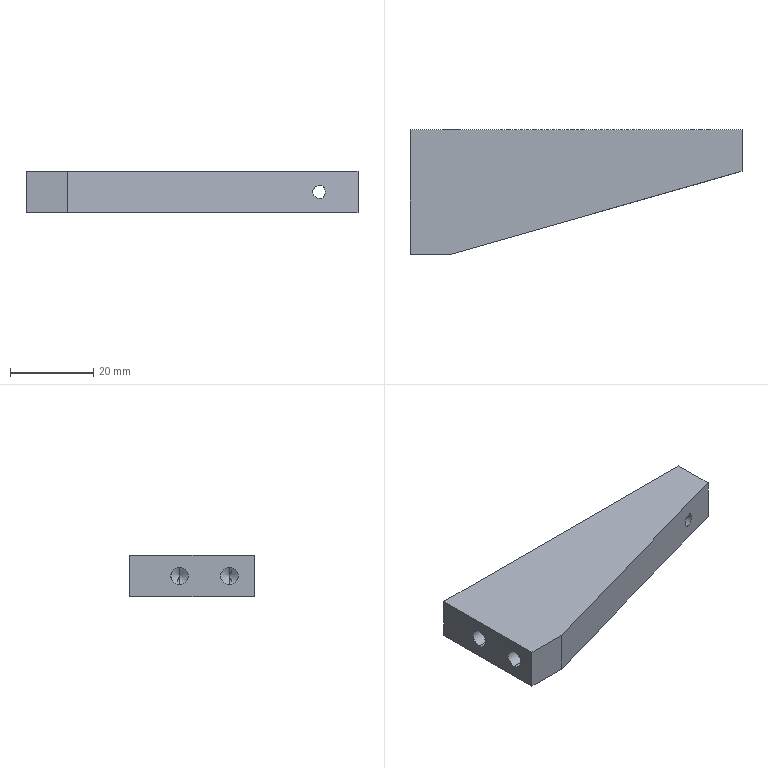Part | NX | features BREP 1 | 1 solid | 33 faces | box 80 x 30 x 10 mm | volume 16150 mm3 | cylinder 14 | cone 12 | plane 7 | commonest cylinder face diameters 4.2 x14
STEP:
#1=CARTESIAN_POINT('',(-30.,2.6,7.1));
#2=VERTEX_POINT('',#1);
#3=CARTESIAN_POINT('',(-29.6,2.6,7.062));
#4=VERTEX_POINT('',#3);
#5=CARTESIAN_POINT('',(-30.,2.6,5.));
#6=DIRECTION('',(0.,1.,0.));
#7=DIRECTION('',(0.,0.,1.));
#8=AXIS2_PLACEMENT_3D('',#5,#6,#7);
#9=CIRCLE('',#8,2.1);
#10=EDGE_CURVE('',#2,#4,#9,.T.);
#11=ORIENTED_EDGE('',*,*,#10,.F.);
#12=CARTESIAN_POINT('',(-30.,3.,7.1));
#13=VERTEX_POINT('',#12);
#14=CARTESIAN_POINT('',(-30.,15.,7.1));
#15=DIRECTION('',(0.,1.,0.));
#16=VECTOR('',#15,1000.);
#17=LINE('',#14,#16);
#18=EDGE_CURVE('',#2,#13,#17,.T.);
#19=ORIENTED_EDGE('',*,*,#18,.T.);
#20=CARTESIAN_POINT('',(-30.,3.,7.1));
#21=CARTESIAN_POINT('',(-29.866,2.866,7.1));
#22=CARTESIAN_POINT('',(-29.732,2.732,7.087));
#23=CARTESIAN_POINT('',(-29.6,2.6,7.062));
#24=(BOUNDED_CURVE()B_SPLINE_CURVE(3,(#20,#21,#22,#23),.UNSPECIFIED.,.F.,.F.)B_SPLINE_CURVE_WITH_KNOTS((4,4),(1.571,1.762),.UNSPECIFIED.)CURVE()GEOMETRIC_REPRESENTATION_ITEM()RATIONAL_B_SPLINE_CURVE((1.,0.9969,0.9969,1.))REPRESENTATION_ITEM(''));
#25=EDGE_CURVE('',#13,#4,#24,.T.);
#26=ORIENTED_EDGE('',*,*,#25,.T.);
#27=EDGE_LOOP('',(#11,#19,#26));
#28=FACE_BOUND('',#27,.T.);
#29=CARTESIAN_POINT('',(-30.,15.,5.));
#30=DIRECTION('',(0.,1.,0.));
#31=DIRECTION('',(0.,0.,1.));
#32=AXIS2_PLACEMENT_3D('',#29,#30,#31);
#33=CYLINDRICAL_SURFACE('',#32,2.1);
#34=ADVANCED_FACE('',(#28),#33,.F.);
#35=CARTESIAN_POINT('',(-30.,2.574,7.056));
#36=VERTEX_POINT('',#35);
#37=CARTESIAN_POINT('',(-30.,2.574,7.056));
#38=CARTESIAN_POINT('',(-29.869,2.574,7.056));
#39=CARTESIAN_POINT('',(-29.735,2.583,7.058));
#40=CARTESIAN_POINT('',(-29.6,2.6,7.062));
#41=B_SPLINE_CURVE_WITH_KNOTS('',3,(#37,#38,#39,#40),.UNSPECIFIED.,.F.,.F.,(4,4),(0.,1.),.UNSPECIFIED.);
#42=EDGE_CURVE('',#4,#36,#41,.F.);
#43=ORIENTED_EDGE('',*,*,#42,.T.);
#44=CARTESIAN_POINT('',(-30.,2.6,7.1));
#45=DIRECTION('',(0.,0.515,0.8572));
#46=VECTOR('',#45,1000.);
#47=LINE('',#44,#46);
#48=EDGE_CURVE('',#36,#2,#47,.T.);
#49=ORIENTED_EDGE('',*,*,#48,.T.);
#50=ORIENTED_EDGE('',*,*,#10,.T.);
#51=EDGE_LOOP('',(#43,#49,#50));
#52=FACE_BOUND('',#51,.T.);
#53=CARTESIAN_POINT('',(-30.,2.6,5.));
#54=DIRECTION('',(0.,1.,0.));
#55=DIRECTION('',(0.,0.,1.));
#56=AXIS2_PLACEMENT_3D('',#53,#54,#55);
#57=CONICAL_SURFACE('',#56,2.1,1.03);
#58=ADVANCED_FACE('',(#52),#57,.F.);
#59=CARTESIAN_POINT('',(-27.6,3.,7.1));
#60=VERTEX_POINT('',#59);
#61=CARTESIAN_POINT('',(-26.338,3.,5.));
#62=VERTEX_POINT('',#61);
#63=CARTESIAN_POINT('',(-27.6,3.,7.1));
#64=DIRECTION('',(-0.515,0.,0.8572));
#65=VECTOR('',#64,1000.);
#66=LINE('',#63,#65);
#67=EDGE_CURVE('',#60,#62,#66,.F.);
#68=ORIENTED_EDGE('',*,*,#67,.T.);
#69=CARTESIAN_POINT('',(-27.6,3.,2.9));
#70=VERTEX_POINT('',#69);
#71=CARTESIAN_POINT('',(-27.6,3.,2.9));
#72=DIRECTION('',(-0.515,0.,-0.8572));
#73=VECTOR('',#72,1000.);
#74=LINE('',#71,#73);
#75=EDGE_CURVE('',#70,#62,#74,.F.);
#76=ORIENTED_EDGE('',*,*,#75,.F.);
#77=CARTESIAN_POINT('',(-27.6,3.,5.));
#78=DIRECTION('',(-1.,0.,0.));
#79=DIRECTION('',(0.,0.,1.));
#80=AXIS2_PLACEMENT_3D('',#77,#78,#79);
#81=CIRCLE('',#80,2.1);
#82=EDGE_CURVE('',#70,#60,#81,.T.);
#83=ORIENTED_EDGE('',*,*,#82,.T.);
#84=EDGE_LOOP('',(#68,#76,#83));
#85=FACE_BOUND('',#84,.T.);
#86=CARTESIAN_POINT('',(-27.6,3.,5.));
#87=DIRECTION('',(-1.,0.,0.));
#88=DIRECTION('',(0.,0.,1.));
#89=AXIS2_PLACEMENT_3D('',#86,#87,#88);
#90=CONICAL_SURFACE('',#89,2.1,1.03);
#91=ADVANCED_FACE('',(#85),#90,.F.);
#92=ORIENTED_EDGE('',*,*,#82,.F.);
#93=CARTESIAN_POINT('',(-30.,3.,2.9));
#94=VERTEX_POINT('',#93);
#95=CARTESIAN_POINT('',(-40.,3.,2.9));
#96=DIRECTION('',(-1.,0.,0.));
#97=VECTOR('',#96,1000.);
#98=LINE('',#95,#97);
#99=EDGE_CURVE('',#94,#70,#98,.F.);
#100=ORIENTED_EDGE('',*,*,#99,.F.);
#101=CARTESIAN_POINT('',(-29.6,2.6,2.938));
#102=VERTEX_POINT('',#101);
#103=CARTESIAN_POINT('',(-29.6,2.6,2.938));
#104=CARTESIAN_POINT('',(-29.732,2.732,2.913));
#105=CARTESIAN_POINT('',(-29.866,2.866,2.9));
#106=CARTESIAN_POINT('',(-30.,3.,2.9));
#107=(BOUNDED_CURVE()B_SPLINE_CURVE(3,(#103,#104,#105,#106),.UNSPECIFIED.,.F.,.F.)B_SPLINE_CURVE_WITH_KNOTS((4,4),(4.521,4.712),.UNSPECIFIED.)CURVE()GEOMETRIC_REPRESENTATION_ITEM()RATIONAL_B_SPLINE_CURVE((1.,0.9969,0.9969,1.))REPRESENTATION_ITEM(''));
#108=EDGE_CURVE('',#102,#94,#107,.T.);
#109=ORIENTED_EDGE('',*,*,#108,.F.);
#110=CARTESIAN_POINT('',(-30.4,2.6,2.938));
#111=VERTEX_POINT('',#110);
#112=CARTESIAN_POINT('',(-29.6,2.6,2.938));
#113=CARTESIAN_POINT('',(-29.872,2.565,2.945));
#114=CARTESIAN_POINT('',(-30.129,2.565,2.945));
#115=CARTESIAN_POINT('',(-30.4,2.6,2.938));
#116=B_SPLINE_CURVE_WITH_KNOTS('',3,(#112,#113,#114,#115),.UNSPECIFIED.,.F.,.F.,(4,4),(0.,1.),.UNSPECIFIED.);
#117=EDGE_CURVE('',#111,#102,#116,.F.);
#118=ORIENTED_EDGE('',*,*,#117,.F.);
#119=CARTESIAN_POINT('',(-30.,3.,2.9));
#120=CARTESIAN_POINT('',(-30.134,2.866,2.9));
#121=CARTESIAN_POINT('',(-30.268,2.732,2.913));
#122=CARTESIAN_POINT('',(-30.4,2.6,2.938));
#123=(BOUNDED_CURVE()B_SPLINE_CURVE(3,(#119,#120,#121,#122),.UNSPECIFIED.,.F.,.F.)B_SPLINE_CURVE_WITH_KNOTS((4,4),(1.571,1.762),.UNSPECIFIED.)CURVE()GEOMETRIC_REPRESENTATION_ITEM()RATIONAL_B_SPLINE_CURVE((1.,0.9969,0.9969,1.))REPRESENTATION_ITEM(''));
#124=EDGE_CURVE('',#94,#111,#123,.T.);
#125=ORIENTED_EDGE('',*,*,#124,.F.);
#126=CARTESIAN_POINT('',(-40.,3.,2.9));
#127=VERTEX_POINT('',#126);
#128=CARTESIAN_POINT('',(-40.,3.,2.9));
#129=DIRECTION('',(-1.,0.,0.));
#130=VECTOR('',#129,1000.);
#131=LINE('',#128,#130);
#132=EDGE_CURVE('',#127,#94,#131,.F.);
#133=ORIENTED_EDGE('',*,*,#132,.F.);
#134=CARTESIAN_POINT('',(-40.,3.,7.1));
#135=VERTEX_POINT('',#134);
#136=CARTESIAN_POINT('',(-40.,3.,5.));
#137=DIRECTION('',(-1.,0.,0.));
#138=DIRECTION('',(0.,0.,1.));
#139=AXIS2_PLACEMENT_3D('',#136,#137,#138);
#140=CIRCLE('',#139,2.1);
#141=EDGE_CURVE('',#127,#135,#140,.T.);
#142=ORIENTED_EDGE('',*,*,#141,.T.);
#143=CARTESIAN_POINT('',(-40.,3.,7.1));
#144=DIRECTION('',(-1.,0.,0.));
#145=VECTOR('',#144,1000.);
#146=LINE('',#143,#145);
#147=EDGE_CURVE('',#135,#13,#146,.F.);
#148=ORIENTED_EDGE('',*,*,#147,.T.);
#149=CARTESIAN_POINT('',(-30.4,2.6,7.062));
#150=VERTEX_POINT('',#149);
#151=CARTESIAN_POINT('',(-30.4,2.6,7.062));
#152=CARTESIAN_POINT('',(-30.268,2.732,7.087));
#153=CARTESIAN_POINT('',(-30.134,2.866,7.1));
#154=CARTESIAN_POINT('',(-30.,3.,7.1));
#155=(BOUNDED_CURVE()B_SPLINE_CURVE(3,(#151,#152,#153,#154),.UNSPECIFIED.,.F.,.F.)B_SPLINE_CURVE_WITH_KNOTS((4,4),(4.521,4.712),.UNSPECIFIED.)CURVE()GEOMETRIC_REPRESENTATION_ITEM()RATIONAL_B_SPLINE_CURVE((1.,0.9969,0.9969,1.))REPRESENTATION_ITEM(''));
#156=EDGE_CURVE('',#150,#13,#155,.T.);
#157=ORIENTED_EDGE('',*,*,#156,.F.);
#158=CARTESIAN_POINT('',(-30.4,2.6,7.062));
#159=CARTESIAN_POINT('',(-30.265,2.583,7.058));
#160=CARTESIAN_POINT('',(-30.131,2.574,7.056));
#161=CARTESIAN_POINT('',(-30.,2.574,7.056));
#162=B_SPLINE_CURVE_WITH_KNOTS('',3,(#158,#159,#160,#161),.UNSPECIFIED.,.F.,.F.,(4,4),(0.,1.),.UNSPECIFIED.);
#163=EDGE_CURVE('',#36,#150,#162,.F.);
#164=ORIENTED_EDGE('',*,*,#163,.F.);
#165=ORIENTED_EDGE('',*,*,#42,.F.);
#166=ORIENTED_EDGE('',*,*,#25,.F.);
#167=CARTESIAN_POINT('',(-40.,3.,7.1));
#168=DIRECTION('',(-1.,0.,0.));
#169=VECTOR('',#168,1000.);
#170=LINE('',#167,#169);
#171=EDGE_CURVE('',#13,#60,#170,.F.);
#172=ORIENTED_EDGE('',*,*,#171,.T.);
#173=EDGE_LOOP('',(#92,#100,#109,#118,#125,#133,#142,#148,#157,#164,#165,#166,#172));
#174=FACE_BOUND('',#173,.T.);
#175=CARTESIAN_POINT('',(-40.,3.,5.));
#176=DIRECTION('',(-1.,0.,0.));
#177=DIRECTION('',(0.,0.,1.));
#178=AXIS2_PLACEMENT_3D('',#175,#176,#177);
#179=CYLINDRICAL_SURFACE('',#178,2.1);
#180=ADVANCED_FACE('',(#174),#179,.F.);
#181=ORIENTED_EDGE('',*,*,#99,.T.);
#182=CARTESIAN_POINT('',(-27.6,3.,5.));
#183=DIRECTION('',(-1.,0.,0.));
#184=DIRECTION('',(0.,0.,1.));
#185=AXIS2_PLACEMENT_3D('',#182,#183,#184);
#186=CIRCLE('',#185,2.1);
#187=EDGE_CURVE('',#60,#70,#186,.T.);
#188=ORIENTED_EDGE('',*,*,#187,.F.);
#189=ORIENTED_EDGE('',*,*,#171,.F.);
#190=CARTESIAN_POINT('',(-30.,3.,2.9));
#191=CARTESIAN_POINT('',(-25.8,7.2,2.9));
#192=CARTESIAN_POINT('',(-25.8,7.2,7.1));
#193=CARTESIAN_POINT('',(-30.,3.,7.1));
#194=(BOUNDED_CURVE()B_SPLINE_CURVE(3,(#190,#191,#192,#193),.UNSPECIFIED.,.F.,.F.)B_SPLINE_CURVE_WITH_KNOTS((4,4),(4.712,7.854),.UNSPECIFIED.)CURVE()GEOMETRIC_REPRESENTATION_ITEM()RATIONAL_B_SPLINE_CURVE((1.,0.3333,0.3333,1.))REPRESENTATION_ITEM(''));
#195=EDGE_CURVE('',#94,#13,#194,.T.);
#196=ORIENTED_EDGE('',*,*,#195,.F.);
#197=EDGE_LOOP('',(#181,#188,#189,#196));
#198=FACE_BOUND('',#197,.T.);
#199=CARTESIAN_POINT('',(-40.,3.,5.));
#200=DIRECTION('',(-1.,0.,0.));
#201=DIRECTION('',(0.,0.,1.));
#202=AXIS2_PLACEMENT_3D('',#199,#200,#201);
#203=CYLINDRICAL_SURFACE('',#202,2.1);
#204=ADVANCED_FACE('',(#198),#203,.F.);
#205=CARTESIAN_POINT('',(-27.6,-9.,2.9));
#206=VERTEX_POINT('',#205);
#207=CARTESIAN_POINT('',(-27.6,-9.,7.1));
#208=VERTEX_POINT('',#207);
#209=CARTESIAN_POINT('',(-27.6,-9.,5.));
#210=DIRECTION('',(-1.,0.,0.));
#211=DIRECTION('',(0.,0.,1.));
#212=AXIS2_PLACEMENT_3D('',#209,#210,#211);
#213=CIRCLE('',#212,2.1);
#214=EDGE_CURVE('',#206,#208,#213,.T.);
#215=ORIENTED_EDGE('',*,*,#214,.F.);
#216=CARTESIAN_POINT('',(-40.,-9.,2.9));
#217=VERTEX_POINT('',#216);
#218=CARTESIAN_POINT('',(-40.,-9.,2.9));
#219=DIRECTION('',(-1.,0.,0.));
#220=VECTOR('',#219,1000.);
#221=LINE('',#218,#220);
#222=EDGE_CURVE('',#217,#206,#221,.F.);
#223=ORIENTED_EDGE('',*,*,#222,.F.);
#224=CARTESIAN_POINT('',(-40.,-9.,7.1));
#225=VERTEX_POINT('',#224);
#226=CARTESIAN_POINT('',(-40.,-9.,5.));
#227=DIRECTION('',(-1.,0.,0.));
#228=DIRECTION('',(0.,0.,1.));
#229=AXIS2_PLACEMENT_3D('',#226,#227,#228);
#230=CIRCLE('',#229,2.1);
#231=EDGE_CURVE('',#217,#225,#230,.T.);
#232=ORIENTED_EDGE('',*,*,#231,.T.);
#233=CARTESIAN_POINT('',(-40.,-9.,7.1));
#234=DIRECTION('',(-1.,0.,0.));
#235=VECTOR('',#234,1000.);
#236=LINE('',#233,#235);
#237=EDGE_CURVE('',#225,#208,#236,.F.);
#238=ORIENTED_EDGE('',*,*,#237,.T.);
#239=EDGE_LOOP('',(#215,#223,#232,#238));
#240=FACE_BOUND('',#239,.T.);
#241=CARTESIAN_POINT('',(-40.,-9.,5.));
#242=DIRECTION('',(-1.,0.,0.));
#243=DIRECTION('',(0.,0.,1.));
#244=AXIS2_PLACEMENT_3D('',#241,#242,#243);
#245=CYLINDRICAL_SURFACE('',#244,2.1);
#246=ADVANCED_FACE('',(#240),#245,.F.);
#247=CARTESIAN_POINT('',(-26.338,-9.,5.));
#248=VERTEX_POINT('',#247);
#249=CARTESIAN_POINT('',(-27.6,-9.,7.1));
#250=DIRECTION('',(-0.515,0.,0.8572));
#251=VECTOR('',#250,1000.);
#252=LINE('',#249,#251);
#253=EDGE_CURVE('',#208,#248,#252,.F.);
#254=ORIENTED_EDGE('',*,*,#253,.T.);
#255=CARTESIAN_POINT('',(-27.6,-9.,2.9));
#256=DIRECTION('',(-0.515,0.,-0.8572));
#257=VECTOR('',#256,1000.);
#258=LINE('',#255,#257);
#259=EDGE_CURVE('',#206,#248,#258,.F.);
#260=ORIENTED_EDGE('',*,*,#259,.F.);
#261=ORIENTED_EDGE('',*,*,#214,.T.);
#262=EDGE_LOOP('',(#254,#260,#261));
#263=FACE_BOUND('',#262,.T.);
#264=CARTESIAN_POINT('',(-27.6,-9.,5.));
#265=DIRECTION('',(-1.,0.,0.));
#266=DIRECTION('',(0.,0.,1.));
#267=AXIS2_PLACEMENT_3D('',#264,#265,#266);
#268=CONICAL_SURFACE('',#267,2.1,1.03);
#269=ADVANCED_FACE('',(#263),#268,.F.);
#270=CARTESIAN_POINT('',(0.,2.6,2.9));
#271=VERTEX_POINT('',#270);
#272=CARTESIAN_POINT('',(0.,2.6,7.1));
#273=VERTEX_POINT('',#272);
#274=CARTESIAN_POINT('',(0.,2.6,5.));
#275=DIRECTION('',(0.,1.,0.));
#276=DIRECTION('',(0.,0.,1.));
#277=AXIS2_PLACEMENT_3D('',#274,#275,#276);
#278=CIRCLE('',#277,2.1);
#279=EDGE_CURVE('',#271,#273,#278,.T.);
#280=ORIENTED_EDGE('',*,*,#279,.F.);
#281=CARTESIAN_POINT('',(0.,15.,2.9));
#282=VERTEX_POINT('',#281);
#283=CARTESIAN_POINT('',(0.,15.,2.9));
#284=DIRECTION('',(0.,1.,0.));
#285=VECTOR('',#284,1000.);
#286=LINE('',#283,#285);
#287=EDGE_CURVE('',#282,#271,#286,.F.);
#288=ORIENTED_EDGE('',*,*,#287,.F.);
#289=CARTESIAN_POINT('',(0.,15.,7.1));
#290=VERTEX_POINT('',#289);
#291=CARTESIAN_POINT('',(0.,15.,5.));
#292=DIRECTION('',(0.,1.,0.));
#293=DIRECTION('',(0.,0.,1.));
#294=AXIS2_PLACEMENT_3D('',#291,#292,#293);
#295=CIRCLE('',#294,2.1);
#296=EDGE_CURVE('',#282,#290,#295,.T.);
#297=ORIENTED_EDGE('',*,*,#296,.T.);
#298=CARTESIAN_POINT('',(0.,15.,7.1));
#299=DIRECTION('',(0.,1.,0.));
#300=VECTOR('',#299,1000.);
#301=LINE('',#298,#300);
#302=EDGE_CURVE('',#290,#273,#301,.F.);
#303=ORIENTED_EDGE('',*,*,#302,.T.);
#304=EDGE_LOOP('',(#280,#288,#297,#303));
#305=FACE_BOUND('',#304,.T.);
#306=CARTESIAN_POINT('',(0.,15.,5.));
#307=DIRECTION('',(0.,1.,0.));
#308=DIRECTION('',(0.,0.,1.));
#309=AXIS2_PLACEMENT_3D('',#306,#307,#308);
#310=CYLINDRICAL_SURFACE('',#309,2.1);
#311=ADVANCED_FACE('',(#305),#310,.F.);
#312=CARTESIAN_POINT('',(0.,1.338,5.));
#313=VERTEX_POINT('',#312);
#314=CARTESIAN_POINT('',(0.,2.6,7.1));
#315=DIRECTION('',(0.,0.515,0.8572));
#316=VECTOR('',#315,1000.);
#317=LINE('',#314,#316);
#318=EDGE_CURVE('',#273,#313,#317,.F.);
#319=ORIENTED_EDGE('',*,*,#318,.T.);
#320=CARTESIAN_POINT('',(0.,2.6,2.9));
#321=DIRECTION('',(0.,0.515,-0.8572));
#322=VECTOR('',#321,1000.);
#323=LINE('',#320,#322);
#324=EDGE_CURVE('',#271,#313,#323,.F.);
#325=ORIENTED_EDGE('',*,*,#324,.F.);
#326=ORIENTED_EDGE('',*,*,#279,.T.);
#327=EDGE_LOOP('',(#319,#325,#326));
#328=FACE_BOUND('',#327,.T.);
#329=CARTESIAN_POINT('',(0.,2.6,5.));
#330=DIRECTION('',(0.,1.,0.));
#331=DIRECTION('',(0.,0.,1.));
#332=AXIS2_PLACEMENT_3D('',#329,#330,#331);
#333=CONICAL_SURFACE('',#332,2.1,1.03);
#334=ADVANCED_FACE('',(#328),#333,.F.);
#335=CARTESIAN_POINT('',(30.,2.6,2.9));
#336=VERTEX_POINT('',#335);
#337=CARTESIAN_POINT('',(30.,2.6,7.1));
#338=VERTEX_POINT('',#337);
#339=CARTESIAN_POINT('',(30.,2.6,5.));
#340=DIRECTION('',(0.,1.,0.));
#341=DIRECTION('',(0.,0.,1.));
#342=AXIS2_PLACEMENT_3D('',#339,#340,#341);
#343=CIRCLE('',#342,2.1);
#344=EDGE_CURVE('',#336,#338,#343,.T.);
#345=ORIENTED_EDGE('',*,*,#344,.F.);
#346=CARTESIAN_POINT('',(30.,15.,2.9));
#347=VERTEX_POINT('',#346);
#348=CARTESIAN_POINT('',(30.,15.,2.9));
#349=DIRECTION('',(0.,1.,0.));
#350=VECTOR('',#349,1000.);
#351=LINE('',#348,#350);
#352=EDGE_CURVE('',#347,#336,#351,.F.);
#353=ORIENTED_EDGE('',*,*,#352,.F.);
#354=CARTESIAN_POINT('',(30.,15.,7.1));
#355=VERTEX_POINT('',#354);
#356=CARTESIAN_POINT('',(30.,15.,5.));
#357=DIRECTION('',(0.,1.,0.));
#358=DIRECTION('',(0.,0.,1.));
#359=AXIS2_PLACEMENT_3D('',#356,#357,#358);
#360=CIRCLE('',#359,2.1);
#361=EDGE_CURVE('',#347,#355,#360,.T.);
#362=ORIENTED_EDGE('',*,*,#361,.T.);
#363=CARTESIAN_POINT('',(30.,15.,7.1));
#364=DIRECTION('',(0.,1.,0.));
#365=VECTOR('',#364,1000.);
#366=LINE('',#363,#365);
#367=EDGE_CURVE('',#355,#338,#366,.F.);
#368=ORIENTED_EDGE('',*,*,#367,.T.);
#369=EDGE_LOOP('',(#345,#353,#362,#368));
#370=FACE_BOUND('',#369,.T.);
#371=CARTESIAN_POINT('',(30.,15.,5.));
#372=DIRECTION('',(0.,1.,0.));
#373=DIRECTION('',(0.,0.,1.));
#374=AXIS2_PLACEMENT_3D('',#371,#372,#373);
#375=CYLINDRICAL_SURFACE('',#374,2.1);
#376=ADVANCED_FACE('',(#370),#375,.F.);
#377=CARTESIAN_POINT('',(30.,2.143,3.661));
#378=VERTEX_POINT('',#377);
#379=CARTESIAN_POINT('',(30.,2.143,6.339));
#380=VERTEX_POINT('',#379);
#381=CARTESIAN_POINT('',(30.,2.143,3.661));
#382=CARTESIAN_POINT('',(28.627,1.751,4.314));
#383=CARTESIAN_POINT('',(28.627,1.751,5.686));
#384=CARTESIAN_POINT('',(30.,2.143,6.339));
#385=(BOUNDED_CURVE()B_SPLINE_CURVE(3,(#381,#382,#383,#384),.UNSPECIFIED.,.F.,.F.)B_SPLINE_CURVE_WITH_KNOTS((4,4),(2.066,4.217),.UNSPECIFIED.)CURVE()GEOMETRIC_REPRESENTATION_ITEM()RATIONAL_B_SPLINE_CURVE((1.,0.6503,0.6503,1.))REPRESENTATION_ITEM(''));
#386=EDGE_CURVE('',#378,#380,#385,.T.);
#387=ORIENTED_EDGE('',*,*,#386,.F.);
#388=CARTESIAN_POINT('',(30.,2.6,2.9));
#389=DIRECTION('',(0.,0.515,-0.8572));
#390=VECTOR('',#389,1000.);
#391=LINE('',#388,#390);
#392=EDGE_CURVE('',#378,#336,#391,.T.);
#393=ORIENTED_EDGE('',*,*,#392,.T.);
#394=ORIENTED_EDGE('',*,*,#344,.T.);
#395=CARTESIAN_POINT('',(30.,2.6,7.1));
#396=DIRECTION('',(0.,0.515,0.8572));
#397=VECTOR('',#396,1000.);
#398=LINE('',#395,#397);
#399=EDGE_CURVE('',#380,#338,#398,.T.);
#400=ORIENTED_EDGE('',*,*,#399,.F.);
#401=EDGE_LOOP('',(#387,#393,#394,#400));
#402=FACE_BOUND('',#401,.T.);
#403=CARTESIAN_POINT('',(30.,2.6,5.));
#404=DIRECTION('',(0.,1.,0.));
#405=DIRECTION('',(0.,0.,1.));
#406=AXIS2_PLACEMENT_3D('',#403,#404,#405);
#407=CONICAL_SURFACE('',#406,2.1,1.03);
#408=ADVANCED_FACE('',(#402),#407,.F.);
#409=CARTESIAN_POINT('',(31.6,2.6,6.36));
#410=VERTEX_POINT('',#409);
#411=CARTESIAN_POINT('',(30.,2.143,6.339));
#412=CARTESIAN_POINT('',(30.508,2.288,6.581));
#413=CARTESIAN_POINT('',(31.084,2.453,6.588));
#414=CARTESIAN_POINT('',(31.6,2.6,6.36));
#415=(BOUNDED_CURVE()B_SPLINE_CURVE(3,(#411,#412,#413,#414),.UNSPECIFIED.,.F.,.F.)B_SPLINE_CURVE_WITH_KNOTS((4,4),(4.217,5.178),.UNSPECIFIED.)CURVE()GEOMETRIC_REPRESENTATION_ITEM()RATIONAL_B_SPLINE_CURVE((1.,0.9245,0.9245,1.))REPRESENTATION_ITEM(''));
#416=EDGE_CURVE('',#380,#410,#415,.T.);
#417=ORIENTED_EDGE('',*,*,#416,.F.);
#418=ORIENTED_EDGE('',*,*,#399,.T.);
#419=CARTESIAN_POINT('',(30.,2.6,5.));
#420=DIRECTION('',(0.,1.,0.));
#421=DIRECTION('',(0.,0.,1.));
#422=AXIS2_PLACEMENT_3D('',#419,#420,#421);
#423=CIRCLE('',#422,2.1);
#424=EDGE_CURVE('',#338,#410,#423,.T.);
#425=ORIENTED_EDGE('',*,*,#424,.T.);
#426=EDGE_LOOP('',(#417,#418,#425));
#427=FACE_BOUND('',#426,.T.);
#428=CARTESIAN_POINT('',(30.,2.6,5.));
#429=DIRECTION('',(0.,1.,0.));
#430=DIRECTION('',(0.,0.,1.));
#431=AXIS2_PLACEMENT_3D('',#428,#429,#430);
#432=CONICAL_SURFACE('',#431,2.1,1.03);
#433=ADVANCED_FACE('',(#427),#432,.F.);
#434=CARTESIAN_POINT('',(-30.,3.,7.1));
#435=CARTESIAN_POINT('',(-34.2,7.2,7.1));
#436=CARTESIAN_POINT('',(-34.2,7.2,2.9));
#437=CARTESIAN_POINT('',(-30.,3.,2.9));
#438=(BOUNDED_CURVE()B_SPLINE_CURVE(3,(#434,#435,#436,#437),.UNSPECIFIED.,.F.,.F.)B_SPLINE_CURVE_WITH_KNOTS((4,4),(4.712,7.854),.UNSPECIFIED.)CURVE()GEOMETRIC_REPRESENTATION_ITEM()RATIONAL_B_SPLINE_CURVE((1.,0.3333,0.3333,1.))REPRESENTATION_ITEM(''));
#439=EDGE_CURVE('',#13,#94,#438,.T.);
#440=ORIENTED_EDGE('',*,*,#439,.T.);
#441=CARTESIAN_POINT('',(-30.,15.,2.9));
#442=VERTEX_POINT('',#441);
#443=CARTESIAN_POINT('',(-30.,15.,2.9));
#444=DIRECTION('',(0.,1.,0.));
#445=VECTOR('',#444,1000.);
#446=LINE('',#443,#445);
#447=EDGE_CURVE('',#442,#94,#446,.F.);
#448=ORIENTED_EDGE('',*,*,#447,.F.);
#449=CARTESIAN_POINT('',(-30.,15.,7.1));
#450=VERTEX_POINT('',#449);
#451=CARTESIAN_POINT('',(-30.,15.,5.));
#452=DIRECTION('',(0.,1.,0.));
#453=DIRECTION('',(0.,0.,1.));
#454=AXIS2_PLACEMENT_3D('',#451,#452,#453);
#455=CIRCLE('',#454,2.1);
#456=EDGE_CURVE('',#442,#450,#455,.T.);
#457=ORIENTED_EDGE('',*,*,#456,.T.);
#458=CARTESIAN_POINT('',(-30.,15.,7.1));
#459=DIRECTION('',(0.,1.,0.));
#460=VECTOR('',#459,1000.);
#461=LINE('',#458,#460);
#462=EDGE_CURVE('',#450,#13,#461,.F.);
#463=ORIENTED_EDGE('',*,*,#462,.T.);
#464=EDGE_LOOP('',(#440,#448,#457,#463));
#465=FACE_BOUND('',#464,.T.);
#466=CARTESIAN_POINT('',(-30.,15.,5.));
#467=DIRECTION('',(0.,1.,0.));
#468=DIRECTION('',(0.,0.,1.));
#469=AXIS2_PLACEMENT_3D('',#466,#467,#468);
#470=CYLINDRICAL_SURFACE('',#469,2.1);
#471=ADVANCED_FACE('',(#465),#470,.F.);
#472=ORIENTED_EDGE('',*,*,#447,.T.);
#473=ORIENTED_EDGE('',*,*,#195,.T.);
#474=ORIENTED_EDGE('',*,*,#462,.F.);
#475=CARTESIAN_POINT('',(-30.,15.,5.));
#476=DIRECTION('',(0.,1.,0.));
#477=DIRECTION('',(0.,0.,1.));
#478=AXIS2_PLACEMENT_3D('',#475,#476,#477);
#479=CIRCLE('',#478,2.1);
#480=EDGE_CURVE('',#450,#442,#479,.T.);
#481=ORIENTED_EDGE('',*,*,#480,.T.);
#482=EDGE_LOOP('',(#472,#473,#474,#481));
#483=FACE_BOUND('',#482,.T.);
#484=CARTESIAN_POINT('',(-30.,15.,5.));
#485=DIRECTION('',(0.,1.,0.));
#486=DIRECTION('',(0.,0.,1.));
#487=AXIS2_PLACEMENT_3D('',#484,#485,#486);
#488=CYLINDRICAL_SURFACE('',#487,2.1);
#489=ADVANCED_FACE('',(#483),#488,.F.);
#490=CARTESIAN_POINT('',(-40.,15.,0.));
#491=VERTEX_POINT('',#490);
#492=CARTESIAN_POINT('',(-40.,-15.,0.));
#493=VERTEX_POINT('',#492);
#494=CARTESIAN_POINT('',(-40.,-15.,0.));
#495=DIRECTION('',(0.,-1.,0.));
#496=VECTOR('',#495,1000.);
#497=LINE('',#494,#496);
#498=EDGE_CURVE('',#491,#493,#497,.T.);
#499=ORIENTED_EDGE('',*,*,#498,.T.);
#500=CARTESIAN_POINT('',(-40.,-15.,10.));
#501=VERTEX_POINT('',#500);
#502=CARTESIAN_POINT('',(-40.,-15.,10.));
#503=DIRECTION('',(0.,0.,-1.));
#504=VECTOR('',#503,1000.);
#505=LINE('',#502,#504);
#506=EDGE_CURVE('',#501,#493,#505,.T.);
#507=ORIENTED_EDGE('',*,*,#506,.F.);
#508=CARTESIAN_POINT('',(-40.,15.,10.));
#509=VERTEX_POINT('',#508);
#510=CARTESIAN_POINT('',(-40.,-15.,10.));
#511=DIRECTION('',(0.,-1.,0.));
#512=VECTOR('',#511,1000.);
#513=LINE('',#510,#512);
#514=EDGE_CURVE('',#509,#501,#513,.T.);
#515=ORIENTED_EDGE('',*,*,#514,.F.);
#516=CARTESIAN_POINT('',(-40.,15.,10.));
#517=DIRECTION('',(0.,0.,-1.));
#518=VECTOR('',#517,1000.);
#519=LINE('',#516,#518);
#520=EDGE_CURVE('',#509,#491,#519,.T.);
#521=ORIENTED_EDGE('',*,*,#520,.T.);
#522=EDGE_LOOP('',(#499,#507,#515,#521));
#523=FACE_BOUND('',#522,.T.);
#524=CARTESIAN_POINT('',(-40.,3.,5.));
#525=DIRECTION('',(-1.,0.,0.));
#526=DIRECTION('',(0.,0.,1.));
#527=AXIS2_PLACEMENT_3D('',#524,#525,#526);
#528=CIRCLE('',#527,2.1);
#529=EDGE_CURVE('',#135,#127,#528,.T.);
#530=ORIENTED_EDGE('',*,*,#529,.F.);
#531=ORIENTED_EDGE('',*,*,#141,.F.);
#532=EDGE_LOOP('',(#530,#531));
#533=FACE_BOUND('',#532,.T.);
#534=CARTESIAN_POINT('',(-40.,-9.,5.));
#535=DIRECTION('',(-1.,0.,0.));
#536=DIRECTION('',(0.,0.,1.));
#537=AXIS2_PLACEMENT_3D('',#534,#535,#536);
#538=CIRCLE('',#537,2.1);
#539=EDGE_CURVE('',#225,#217,#538,.T.);
#540=ORIENTED_EDGE('',*,*,#539,.F.);
#541=ORIENTED_EDGE('',*,*,#231,.F.);
#542=EDGE_LOOP('',(#540,#541));
#543=FACE_BOUND('',#542,.T.);
#544=CARTESIAN_POINT('',(-40.,-15.,10.));
#545=DIRECTION('',(1.,0.,0.));
#546=DIRECTION('',(0.,1.,0.));
#547=AXIS2_PLACEMENT_3D('',#544,#545,#546);
#548=PLANE('',#547);
#549=ADVANCED_FACE('',(#523,#533,#543),#548,.F.);
#550=CARTESIAN_POINT('',(-30.,-15.,0.));
#551=VERTEX_POINT('',#550);
#552=CARTESIAN_POINT('',(-40.,-15.,0.));
#553=DIRECTION('',(1.,0.,0.));
#554=VECTOR('',#553,1000.);
#555=LINE('',#552,#554);
#556=EDGE_CURVE('',#493,#551,#555,.T.);
#557=ORIENTED_EDGE('',*,*,#556,.T.);
#558=CARTESIAN_POINT('',(-30.,-15.,10.));
#559=VERTEX_POINT('',#558);
#560=CARTESIAN_POINT('',(-30.,-15.,10.));
#561=DIRECTION('',(0.,0.,-1.));
#562=VECTOR('',#561,1000.);
#563=LINE('',#560,#562);
#564=EDGE_CURVE('',#559,#551,#563,.T.);
#565=ORIENTED_EDGE('',*,*,#564,.F.);
#566=CARTESIAN_POINT('',(-40.,-15.,10.));
#567=DIRECTION('',(1.,0.,0.));
#568=VECTOR('',#567,1000.);
#569=LINE('',#566,#568);
#570=EDGE_CURVE('',#501,#559,#569,.T.);
#571=ORIENTED_EDGE('',*,*,#570,.F.);
#572=ORIENTED_EDGE('',*,*,#506,.T.);
#573=EDGE_LOOP('',(#557,#565,#571,#572));
#574=FACE_BOUND('',#573,.T.);
#575=CARTESIAN_POINT('',(-40.,-15.,10.));
#576=DIRECTION('',(0.,1.,0.));
#577=DIRECTION('',(1.,0.,0.));
#578=AXIS2_PLACEMENT_3D('',#575,#576,#577);
#579=PLANE('',#578);
#580=ADVANCED_FACE('',(#574),#579,.F.);
#581=CARTESIAN_POINT('',(40.,5.,0.));
#582=VERTEX_POINT('',#581);
#583=CARTESIAN_POINT('',(-30.,-15.,0.));
#584=DIRECTION('',(0.9615,0.2747,0.));
#585=VECTOR('',#584,1000.);
#586=LINE('',#583,#585);
#587=EDGE_CURVE('',#551,#582,#586,.T.);
#588=ORIENTED_EDGE('',*,*,#587,.T.);
#589=CARTESIAN_POINT('',(40.,5.,10.));
#590=VERTEX_POINT('',#589);
#591=CARTESIAN_POINT('',(40.,5.,10.));
#592=DIRECTION('',(0.,0.,-1.));
#593=VECTOR('',#592,1000.);
#594=LINE('',#591,#593);
#595=EDGE_CURVE('',#590,#582,#594,.T.);
#596=ORIENTED_EDGE('',*,*,#595,.F.);
#597=CARTESIAN_POINT('',(-30.,-15.,10.));
#598=DIRECTION('',(0.9615,0.2747,0.));
#599=VECTOR('',#598,1000.);
#600=LINE('',#597,#599);
#601=EDGE_CURVE('',#559,#590,#600,.T.);
#602=ORIENTED_EDGE('',*,*,#601,.F.);
#603=ORIENTED_EDGE('',*,*,#564,.T.);
#604=EDGE_LOOP('',(#588,#596,#602,#603));
#605=FACE_BOUND('',#604,.T.);
#606=CARTESIAN_POINT('',(31.6,2.6,3.64));
#607=VERTEX_POINT('',#606);
#608=CARTESIAN_POINT('',(31.6,2.6,6.36));
#609=CARTESIAN_POINT('',(32.298,2.799,5.539));
#610=CARTESIAN_POINT('',(32.298,2.799,4.461));
#611=CARTESIAN_POINT('',(31.6,2.6,3.64));
#612=(BOUNDED_CURVE()B_SPLINE_CURVE(3,(#608,#609,#610,#611),.UNSPECIFIED.,.F.,.F.)B_SPLINE_CURVE_WITH_KNOTS((4,4),(5.579,6.988),.UNSPECIFIED.)CURVE()GEOMETRIC_REPRESENTATION_ITEM()RATIONAL_B_SPLINE_CURVE((1.,0.8413,0.8413,1.))REPRESENTATION_ITEM(''));
#613=EDGE_CURVE('',#410,#607,#612,.T.);
#614=ORIENTED_EDGE('',*,*,#613,.T.);
#615=CARTESIAN_POINT('',(31.6,2.6,3.64));
#616=CARTESIAN_POINT('',(31.084,2.453,3.412));
#617=CARTESIAN_POINT('',(30.508,2.288,3.419));
#618=CARTESIAN_POINT('',(30.,2.143,3.661));
#619=(BOUNDED_CURVE()B_SPLINE_CURVE(3,(#615,#616,#617,#618),.UNSPECIFIED.,.F.,.F.)B_SPLINE_CURVE_WITH_KNOTS((4,4),(1.105,2.066),.UNSPECIFIED.)CURVE()GEOMETRIC_REPRESENTATION_ITEM()RATIONAL_B_SPLINE_CURVE((1.,0.9245,0.9245,1.))REPRESENTATION_ITEM(''));
#620=EDGE_CURVE('',#607,#378,#619,.T.);
#621=ORIENTED_EDGE('',*,*,#620,.T.);
#622=ORIENTED_EDGE('',*,*,#386,.T.);
#623=ORIENTED_EDGE('',*,*,#416,.T.);
#624=EDGE_LOOP('',(#614,#621,#622,#623));
#625=FACE_BOUND('',#624,.T.);
#626=CARTESIAN_POINT('',(-30.,-15.,10.));
#627=DIRECTION('',(-0.2747,0.9615,0.));
#628=DIRECTION('',(0.,0.,1.));
#629=AXIS2_PLACEMENT_3D('',#626,#627,#628);
#630=PLANE('',#629);
#631=ADVANCED_FACE('',(#605,#625),#630,.F.);
#632=CARTESIAN_POINT('',(40.,15.,0.));
#633=VERTEX_POINT('',#632);
#634=CARTESIAN_POINT('',(40.,5.,0.));
#635=DIRECTION('',(0.,1.,0.));
#636=VECTOR('',#635,1000.);
#637=LINE('',#634,#636);
#638=EDGE_CURVE('',#582,#633,#637,.T.);
#639=ORIENTED_EDGE('',*,*,#638,.T.);
#640=CARTESIAN_POINT('',(40.,15.,10.));
#641=VERTEX_POINT('',#640);
#642=CARTESIAN_POINT('',(40.,15.,10.));
#643=DIRECTION('',(0.,0.,-1.));
#644=VECTOR('',#643,1000.);
#645=LINE('',#642,#644);
#646=EDGE_CURVE('',#641,#633,#645,.T.);
#647=ORIENTED_EDGE('',*,*,#646,.F.);
#648=CARTESIAN_POINT('',(40.,5.,10.));
#649=DIRECTION('',(0.,1.,0.));
#650=VECTOR('',#649,1000.);
#651=LINE('',#648,#650);
#652=EDGE_CURVE('',#590,#641,#651,.T.);
#653=ORIENTED_EDGE('',*,*,#652,.F.);
#654=ORIENTED_EDGE('',*,*,#595,.T.);
#655=EDGE_LOOP('',(#639,#647,#653,#654));
#656=FACE_BOUND('',#655,.T.);
#657=CARTESIAN_POINT('',(40.,5.,10.));
#658=DIRECTION('',(-1.,0.,0.));
#659=DIRECTION('',(0.,0.,1.));
#660=AXIS2_PLACEMENT_3D('',#657,#658,#659);
#661=PLANE('',#660);
#662=ADVANCED_FACE('',(#656),#661,.F.);
#663=CARTESIAN_POINT('',(-40.,15.,0.));
#664=DIRECTION('',(-1.,0.,0.));
#665=VECTOR('',#664,1000.);
#666=LINE('',#663,#665);
#667=EDGE_CURVE('',#633,#491,#666,.T.);
#668=ORIENTED_EDGE('',*,*,#667,.T.);
#669=ORIENTED_EDGE('',*,*,#520,.F.);
#670=CARTESIAN_POINT('',(-40.,15.,10.));
#671=DIRECTION('',(-1.,0.,0.));
#672=VECTOR('',#671,1000.);
#673=LINE('',#670,#672);
#674=EDGE_CURVE('',#641,#509,#673,.T.);
#675=ORIENTED_EDGE('',*,*,#674,.F.);
#676=ORIENTED_EDGE('',*,*,#646,.T.);
#677=EDGE_LOOP('',(#668,#669,#675,#676));
#678=FACE_BOUND('',#677,.T.);
#679=ORIENTED_EDGE('',*,*,#480,.F.);
#680=ORIENTED_EDGE('',*,*,#456,.F.);
#681=EDGE_LOOP('',(#679,#680));
#682=FACE_BOUND('',#681,.T.);
#683=CARTESIAN_POINT('',(0.,15.,5.));
#684=DIRECTION('',(0.,1.,0.));
#685=DIRECTION('',(0.,0.,1.));
#686=AXIS2_PLACEMENT_3D('',#683,#684,#685);
#687=CIRCLE('',#686,2.1);
#688=EDGE_CURVE('',#290,#282,#687,.T.);
#689=ORIENTED_EDGE('',*,*,#688,.F.);
#690=ORIENTED_EDGE('',*,*,#296,.F.);
#691=EDGE_LOOP('',(#689,#690));
#692=FACE_BOUND('',#691,.T.);
#693=CARTESIAN_POINT('',(30.,15.,5.));
#694=DIRECTION('',(0.,1.,0.));
#695=DIRECTION('',(0.,0.,1.));
#696=AXIS2_PLACEMENT_3D('',#693,#694,#695);
#697=CIRCLE('',#696,2.1);
#698=EDGE_CURVE('',#355,#347,#697,.T.);
#699=ORIENTED_EDGE('',*,*,#698,.F.);
#700=ORIENTED_EDGE('',*,*,#361,.F.);
#701=EDGE_LOOP('',(#699,#700));
#702=FACE_BOUND('',#701,.T.);
#703=CARTESIAN_POINT('',(-40.,15.,10.));
#704=DIRECTION('',(0.,-1.,0.));
#705=DIRECTION('',(0.,0.,-1.));
#706=AXIS2_PLACEMENT_3D('',#703,#704,#705);
#707=PLANE('',#706);
#708=ADVANCED_FACE('',(#678,#682,#692,#702),#707,.F.);
#709=ORIENTED_EDGE('',*,*,#514,.T.);
#710=ORIENTED_EDGE('',*,*,#570,.T.);
#711=ORIENTED_EDGE('',*,*,#601,.T.);
#712=ORIENTED_EDGE('',*,*,#652,.T.);
#713=ORIENTED_EDGE('',*,*,#674,.T.);
#714=EDGE_LOOP('',(#709,#710,#711,#712,#713));
#715=FACE_BOUND('',#714,.T.);
#716=CARTESIAN_POINT('',(-40.,15.,10.));
#717=DIRECTION('',(0.,0.,-1.));
#718=DIRECTION('',(0.,-1.,0.));
#719=AXIS2_PLACEMENT_3D('',#716,#717,#718);
#720=PLANE('',#719);
#721=ADVANCED_FACE('',(#715),#720,.F.);
#722=ORIENTED_EDGE('',*,*,#498,.F.);
#723=ORIENTED_EDGE('',*,*,#667,.F.);
#724=ORIENTED_EDGE('',*,*,#638,.F.);
#725=ORIENTED_EDGE('',*,*,#587,.F.);
#726=ORIENTED_EDGE('',*,*,#556,.F.);
#727=EDGE_LOOP('',(#722,#723,#724,#725,#726));
#728=FACE_BOUND('',#727,.T.);
#729=CARTESIAN_POINT('',(-40.,15.,0.));
#730=DIRECTION('',(0.,0.,-1.));
#731=DIRECTION('',(0.,-1.,0.));
#732=AXIS2_PLACEMENT_3D('',#729,#730,#731);
#733=PLANE('',#732);
#734=ADVANCED_FACE('',(#728),#733,.T.);
#735=ORIENTED_EDGE('',*,*,#392,.F.);
#736=ORIENTED_EDGE('',*,*,#620,.F.);
#737=CARTESIAN_POINT('',(30.,2.6,5.));
#738=DIRECTION('',(0.,1.,0.));
#739=DIRECTION('',(0.,0.,1.));
#740=AXIS2_PLACEMENT_3D('',#737,#738,#739);
#741=CIRCLE('',#740,2.1);
#742=EDGE_CURVE('',#607,#336,#741,.T.);
#743=ORIENTED_EDGE('',*,*,#742,.T.);
#744=EDGE_LOOP('',(#735,#736,#743));
#745=FACE_BOUND('',#744,.T.);
#746=CARTESIAN_POINT('',(30.,2.6,5.));
#747=DIRECTION('',(0.,1.,0.));
#748=DIRECTION('',(0.,0.,1.));
#749=AXIS2_PLACEMENT_3D('',#746,#747,#748);
#750=CONICAL_SURFACE('',#749,2.1,1.03);
#751=ADVANCED_FACE('',(#745),#750,.F.);
#752=ORIENTED_EDGE('',*,*,#352,.T.);
#753=ORIENTED_EDGE('',*,*,#742,.F.);
#754=ORIENTED_EDGE('',*,*,#613,.F.);
#755=ORIENTED_EDGE('',*,*,#424,.F.);
#756=ORIENTED_EDGE('',*,*,#367,.F.);
#757=ORIENTED_EDGE('',*,*,#698,.T.);
#758=EDGE_LOOP('',(#752,#753,#754,#755,#756,#757));
#759=FACE_BOUND('',#758,.T.);
#760=CARTESIAN_POINT('',(30.,15.,5.));
#761=DIRECTION('',(0.,1.,0.));
#762=DIRECTION('',(0.,0.,1.));
#763=AXIS2_PLACEMENT_3D('',#760,#761,#762);
#764=CYLINDRICAL_SURFACE('',#763,2.1);
#765=ADVANCED_FACE('',(#759),#764,.F.);
#766=ORIENTED_EDGE('',*,*,#324,.T.);
#767=ORIENTED_EDGE('',*,*,#318,.F.);
#768=CARTESIAN_POINT('',(0.,2.6,5.));
#769=DIRECTION('',(0.,1.,0.));
#770=DIRECTION('',(0.,0.,1.));
#771=AXIS2_PLACEMENT_3D('',#768,#769,#770);
#772=CIRCLE('',#771,2.1);
#773=EDGE_CURVE('',#273,#271,#772,.T.);
#774=ORIENTED_EDGE('',*,*,#773,.T.);
#775=EDGE_LOOP('',(#766,#767,#774));
#776=FACE_BOUND('',#775,.T.);
#777=CARTESIAN_POINT('',(0.,2.6,5.));
#778=DIRECTION('',(0.,1.,0.));
#779=DIRECTION('',(0.,0.,1.));
#780=AXIS2_PLACEMENT_3D('',#777,#778,#779);
#781=CONICAL_SURFACE('',#780,2.1,1.03);
#782=ADVANCED_FACE('',(#776),#781,.F.);
#783=ORIENTED_EDGE('',*,*,#287,.T.);
#784=ORIENTED_EDGE('',*,*,#773,.F.);
#785=ORIENTED_EDGE('',*,*,#302,.F.);
#786=ORIENTED_EDGE('',*,*,#688,.T.);
#787=EDGE_LOOP('',(#783,#784,#785,#786));
#788=FACE_BOUND('',#787,.T.);
#789=CARTESIAN_POINT('',(0.,15.,5.));
#790=DIRECTION('',(0.,1.,0.));
#791=DIRECTION('',(0.,0.,1.));
#792=AXIS2_PLACEMENT_3D('',#789,#790,#791);
#793=CYLINDRICAL_SURFACE('',#792,2.1);
#794=ADVANCED_FACE('',(#788),#793,.F.);
#795=ORIENTED_EDGE('',*,*,#259,.T.);
#796=ORIENTED_EDGE('',*,*,#253,.F.);
#797=CARTESIAN_POINT('',(-27.6,-9.,5.));
#798=DIRECTION('',(-1.,0.,0.));
#799=DIRECTION('',(0.,0.,1.));
#800=AXIS2_PLACEMENT_3D('',#797,#798,#799);
#801=CIRCLE('',#800,2.1);
#802=EDGE_CURVE('',#208,#206,#801,.T.);
#803=ORIENTED_EDGE('',*,*,#802,.T.);
#804=EDGE_LOOP('',(#795,#796,#803));
#805=FACE_BOUND('',#804,.T.);
#806=CARTESIAN_POINT('',(-27.6,-9.,5.));
#807=DIRECTION('',(-1.,0.,0.));
#808=DIRECTION('',(0.,0.,1.));
#809=AXIS2_PLACEMENT_3D('',#806,#807,#808);
#810=CONICAL_SURFACE('',#809,2.1,1.03);
#811=ADVANCED_FACE('',(#805),#810,.F.);
#812=ORIENTED_EDGE('',*,*,#222,.T.);
#813=ORIENTED_EDGE('',*,*,#802,.F.);
#814=ORIENTED_EDGE('',*,*,#237,.F.);
#815=ORIENTED_EDGE('',*,*,#539,.T.);
#816=EDGE_LOOP('',(#812,#813,#814,#815));
#817=FACE_BOUND('',#816,.T.);
#818=CARTESIAN_POINT('',(-40.,-9.,5.));
#819=DIRECTION('',(-1.,0.,0.));
#820=DIRECTION('',(0.,0.,1.));
#821=AXIS2_PLACEMENT_3D('',#818,#819,#820);
#822=CYLINDRICAL_SURFACE('',#821,2.1);
#823=ADVANCED_FACE('',(#817),#822,.F.);
#824=ORIENTED_EDGE('',*,*,#132,.T.);
#825=ORIENTED_EDGE('',*,*,#439,.F.);
#826=ORIENTED_EDGE('',*,*,#147,.F.);
#827=ORIENTED_EDGE('',*,*,#529,.T.);
#828=EDGE_LOOP('',(#824,#825,#826,#827));
#829=FACE_BOUND('',#828,.T.);
#830=CARTESIAN_POINT('',(-40.,3.,5.));
#831=DIRECTION('',(-1.,0.,0.));
#832=DIRECTION('',(0.,0.,1.));
#833=AXIS2_PLACEMENT_3D('',#830,#831,#832);
#834=CYLINDRICAL_SURFACE('',#833,2.1);
#835=ADVANCED_FACE('',(#829),#834,.F.);
#836=ORIENTED_EDGE('',*,*,#75,.T.);
#837=ORIENTED_EDGE('',*,*,#67,.F.);
#838=ORIENTED_EDGE('',*,*,#187,.T.);
#839=EDGE_LOOP('',(#836,#837,#838));
#840=FACE_BOUND('',#839,.T.);
#841=CARTESIAN_POINT('',(-27.6,3.,5.));
#842=DIRECTION('',(-1.,0.,0.));
#843=DIRECTION('',(0.,0.,1.));
#844=AXIS2_PLACEMENT_3D('',#841,#842,#843);
#845=CONICAL_SURFACE('',#844,2.1,1.03);
#846=ADVANCED_FACE('',(#840),#845,.F.);
#847=ORIENTED_EDGE('',*,*,#48,.F.);
#848=ORIENTED_EDGE('',*,*,#163,.T.);
#849=CARTESIAN_POINT('',(-30.,2.6,5.));
#850=DIRECTION('',(0.,1.,0.));
#851=DIRECTION('',(0.,0.,1.));
#852=AXIS2_PLACEMENT_3D('',#849,#850,#851);
#853=CIRCLE('',#852,2.1);
#854=EDGE_CURVE('',#150,#2,#853,.T.);
#855=ORIENTED_EDGE('',*,*,#854,.T.);
#856=EDGE_LOOP('',(#847,#848,#855));
#857=FACE_BOUND('',#856,.T.);
#858=CARTESIAN_POINT('',(-30.,2.6,5.));
#859=DIRECTION('',(0.,1.,0.));
#860=DIRECTION('',(0.,0.,1.));
#861=AXIS2_PLACEMENT_3D('',#858,#859,#860);
#862=CONICAL_SURFACE('',#861,2.1,1.03);
#863=ADVANCED_FACE('',(#857),#862,.F.);
#864=ORIENTED_EDGE('',*,*,#18,.F.);
#865=ORIENTED_EDGE('',*,*,#854,.F.);
#866=ORIENTED_EDGE('',*,*,#156,.T.);
#867=EDGE_LOOP('',(#864,#865,#866));
#868=FACE_BOUND('',#867,.T.);
#869=CARTESIAN_POINT('',(-30.,15.,5.));
#870=DIRECTION('',(0.,1.,0.));
#871=DIRECTION('',(0.,0.,1.));
#872=AXIS2_PLACEMENT_3D('',#869,#870,#871);
#873=CYLINDRICAL_SURFACE('',#872,2.1);
#874=ADVANCED_FACE('',(#868),#873,.F.);
#875=CARTESIAN_POINT('',(-30.,2.6,5.));
#876=DIRECTION('',(0.,1.,0.));
#877=DIRECTION('',(0.,0.,1.));
#878=AXIS2_PLACEMENT_3D('',#875,#876,#877);
#879=CIRCLE('',#878,2.1);
#880=EDGE_CURVE('',#102,#111,#879,.T.);
#881=ORIENTED_EDGE('',*,*,#880,.T.);
#882=ORIENTED_EDGE('',*,*,#117,.T.);
#883=EDGE_LOOP('',(#881,#882));
#884=FACE_BOUND('',#883,.T.);
#885=CARTESIAN_POINT('',(-30.,2.6,5.));
#886=DIRECTION('',(0.,1.,0.));
#887=DIRECTION('',(0.,0.,1.));
#888=AXIS2_PLACEMENT_3D('',#885,#886,#887);
#889=CONICAL_SURFACE('',#888,2.1,1.03);
#890=ADVANCED_FACE('',(#884),#889,.F.);
#891=ORIENTED_EDGE('',*,*,#108,.T.);
#892=ORIENTED_EDGE('',*,*,#124,.T.);
#893=ORIENTED_EDGE('',*,*,#880,.F.);
#894=EDGE_LOOP('',(#891,#892,#893));
#895=FACE_BOUND('',#894,.T.);
#896=CARTESIAN_POINT('',(-30.,15.,5.));
#897=DIRECTION('',(0.,1.,0.));
#898=DIRECTION('',(0.,0.,1.));
#899=AXIS2_PLACEMENT_3D('',#896,#897,#898);
#900=CYLINDRICAL_SURFACE('',#899,2.1);
#901=ADVANCED_FACE('',(#895),#900,.F.);
#902=CLOSED_SHELL('',(#34,#58,#91,#180,#204,#246,#269,#311,#334,#376,#408,#433,#471,#489,#549,#580,#631,#662,#708,#721,#734,#751,#765,#782,#794,#811,#823,#835,#846,#863,#874,#890,#901));
#903=MANIFOLD_SOLID_BREP('',#902);
#904=(LENGTH_UNIT()NAMED_UNIT(*)SI_UNIT(.MILLI.,.METRE.));
#905=UNCERTAINTY_MEASURE_WITH_UNIT(LENGTH_MEASURE(0.0508),#904,'','');
#906=(NAMED_UNIT(*)PLANE_ANGLE_UNIT()SI_UNIT($,.RADIAN.));
#907=(NAMED_UNIT(*)SI_UNIT($,.STERADIAN.)SOLID_ANGLE_UNIT());
#908=(GEOMETRIC_REPRESENTATION_CONTEXT(3)GLOBAL_UNCERTAINTY_ASSIGNED_CONTEXT((#905))GLOBAL_UNIT_ASSIGNED_CONTEXT((#904,#906,#907))REPRESENTATION_CONTEXT('',''));
#909=ADVANCED_BREP_SHAPE_REPRESENTATION('',(#903),#908);